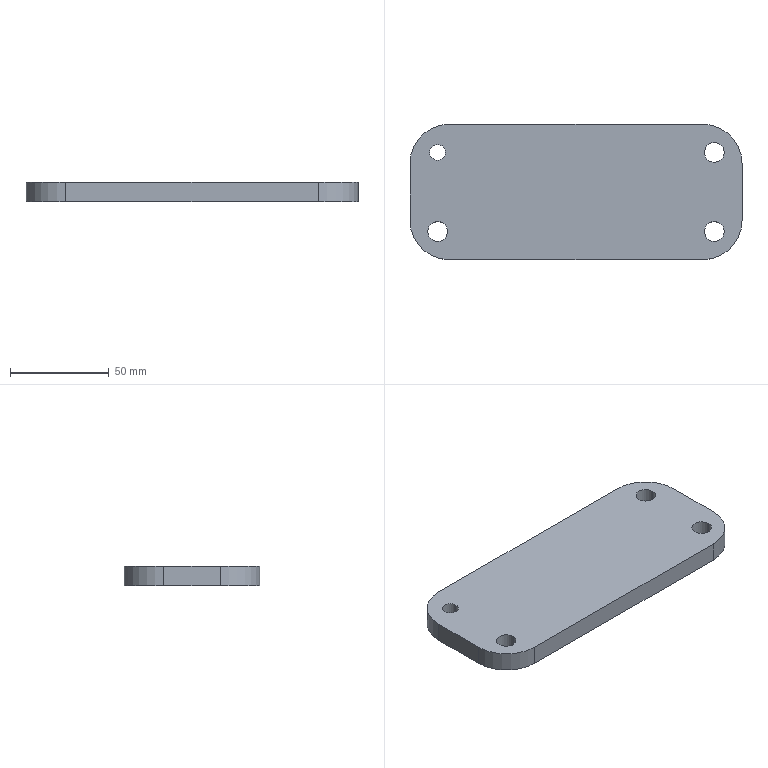Part | SolidWorks | features Cut 1, Extrusion 1, Fillet 1 | 1 solid | 18 faces | box 168 x 68.566 x 10 mm | volume 108898 mm3 | cylinder 12 | plane 6 | commonest cylinder face diameters 10 x6 40 x4 8 x2
STEP:
#1=CARTESIAN_POINT('',(-75.,-100.,-10.));
#2=VERTEX_POINT('',#1);
#3=CARTESIAN_POINT('',(-65.,-100.,-10.));
#4=VERTEX_POINT('',#3);
#5=CARTESIAN_POINT('',(-70.,-100.,-10.));
#6=DIRECTION('',(0.,0.,1.));
#7=DIRECTION('',(1.,0.,0.));
#8=AXIS2_PLACEMENT_3D('',#5,#6,#7);
#9=CIRCLE('',#8,5.);
#10=EDGE_CURVE('',#2,#4,#9,.T.);
#11=ORIENTED_EDGE('',*,*,#10,.F.);
#12=CARTESIAN_POINT('',(-75.,-100.,0.));
#13=VERTEX_POINT('',#12);
#14=CARTESIAN_POINT('',(-75.,-100.,-10.));
#15=DIRECTION('',(0.,0.,1.));
#16=VECTOR('',#15,1000.);
#17=LINE('',#14,#16);
#18=EDGE_CURVE('',#2,#13,#17,.T.);
#19=ORIENTED_EDGE('',*,*,#18,.T.);
#20=CARTESIAN_POINT('',(-65.,-100.,0.));
#21=VERTEX_POINT('',#20);
#22=CARTESIAN_POINT('',(-70.,-100.,0.));
#23=DIRECTION('',(0.,0.,1.));
#24=DIRECTION('',(1.,0.,0.));
#25=AXIS2_PLACEMENT_3D('',#22,#23,#24);
#26=CIRCLE('',#25,5.);
#27=EDGE_CURVE('',#13,#21,#26,.T.);
#28=ORIENTED_EDGE('',*,*,#27,.T.);
#29=CARTESIAN_POINT('',(-65.,-100.,-10.));
#30=DIRECTION('',(0.,0.,1.));
#31=VECTOR('',#30,1000.);
#32=LINE('',#29,#31);
#33=EDGE_CURVE('',#4,#21,#32,.T.);
#34=ORIENTED_EDGE('',*,*,#33,.F.);
#35=EDGE_LOOP('',(#11,#19,#28,#34));
#36=FACE_OUTER_BOUND('',#35,.T.);
#37=CARTESIAN_POINT('',(-70.,-100.,-10.));
#38=DIRECTION('',(0.,0.,1.));
#39=DIRECTION('',(1.,0.,0.));
#40=AXIS2_PLACEMENT_3D('',#37,#38,#39);
#41=CYLINDRICAL_SURFACE('',#40,5.);
#42=ADVANCED_FACE('',(#36),#41,.F.);
#43=CARTESIAN_POINT('',(65.,-60.,-10.));
#44=VERTEX_POINT('',#43);
#45=CARTESIAN_POINT('',(75.,-60.,-10.));
#46=VERTEX_POINT('',#45);
#47=CARTESIAN_POINT('',(70.,-60.,-10.));
#48=DIRECTION('',(0.,0.,1.));
#49=DIRECTION('',(1.,0.,0.));
#50=AXIS2_PLACEMENT_3D('',#47,#48,#49);
#51=CIRCLE('',#50,5.);
#52=EDGE_CURVE('',#44,#46,#51,.T.);
#53=ORIENTED_EDGE('',*,*,#52,.F.);
#54=CARTESIAN_POINT('',(65.,-60.,0.));
#55=VERTEX_POINT('',#54);
#56=CARTESIAN_POINT('',(65.,-60.,-10.));
#57=DIRECTION('',(0.,0.,1.));
#58=VECTOR('',#57,1000.);
#59=LINE('',#56,#58);
#60=EDGE_CURVE('',#44,#55,#59,.T.);
#61=ORIENTED_EDGE('',*,*,#60,.T.);
#62=CARTESIAN_POINT('',(75.,-60.,0.));
#63=VERTEX_POINT('',#62);
#64=CARTESIAN_POINT('',(70.,-60.,0.));
#65=DIRECTION('',(0.,0.,1.));
#66=DIRECTION('',(1.,0.,0.));
#67=AXIS2_PLACEMENT_3D('',#64,#65,#66);
#68=CIRCLE('',#67,5.);
#69=EDGE_CURVE('',#55,#63,#68,.T.);
#70=ORIENTED_EDGE('',*,*,#69,.T.);
#71=CARTESIAN_POINT('',(75.,-60.,-10.));
#72=DIRECTION('',(0.,0.,1.));
#73=VECTOR('',#72,1000.);
#74=LINE('',#71,#73);
#75=EDGE_CURVE('',#46,#63,#74,.T.);
#76=ORIENTED_EDGE('',*,*,#75,.F.);
#77=EDGE_LOOP('',(#53,#61,#70,#76));
#78=FACE_OUTER_BOUND('',#77,.T.);
#79=CARTESIAN_POINT('',(70.,-60.,-10.));
#80=DIRECTION('',(0.,0.,1.));
#81=DIRECTION('',(1.,0.,0.));
#82=AXIS2_PLACEMENT_3D('',#79,#80,#81);
#83=CYLINDRICAL_SURFACE('',#82,5.);
#84=ADVANCED_FACE('',(#78),#83,.F.);
#85=CARTESIAN_POINT('',(65.,-100.,-10.));
#86=VERTEX_POINT('',#85);
#87=CARTESIAN_POINT('',(75.,-100.,-10.));
#88=VERTEX_POINT('',#87);
#89=CARTESIAN_POINT('',(70.,-100.,-10.));
#90=DIRECTION('',(0.,0.,1.));
#91=DIRECTION('',(1.,0.,0.));
#92=AXIS2_PLACEMENT_3D('',#89,#90,#91);
#93=CIRCLE('',#92,5.);
#94=EDGE_CURVE('',#86,#88,#93,.T.);
#95=ORIENTED_EDGE('',*,*,#94,.F.);
#96=CARTESIAN_POINT('',(65.,-100.,0.));
#97=VERTEX_POINT('',#96);
#98=CARTESIAN_POINT('',(65.,-100.,-10.));
#99=DIRECTION('',(0.,0.,1.));
#100=VECTOR('',#99,1000.);
#101=LINE('',#98,#100);
#102=EDGE_CURVE('',#86,#97,#101,.T.);
#103=ORIENTED_EDGE('',*,*,#102,.T.);
#104=CARTESIAN_POINT('',(75.,-100.,0.));
#105=VERTEX_POINT('',#104);
#106=CARTESIAN_POINT('',(70.,-100.,0.));
#107=DIRECTION('',(0.,0.,1.));
#108=DIRECTION('',(1.,0.,0.));
#109=AXIS2_PLACEMENT_3D('',#106,#107,#108);
#110=CIRCLE('',#109,5.);
#111=EDGE_CURVE('',#97,#105,#110,.T.);
#112=ORIENTED_EDGE('',*,*,#111,.T.);
#113=CARTESIAN_POINT('',(75.,-100.,-10.));
#114=DIRECTION('',(0.,0.,1.));
#115=VECTOR('',#114,1000.);
#116=LINE('',#113,#115);
#117=EDGE_CURVE('',#88,#105,#116,.T.);
#118=ORIENTED_EDGE('',*,*,#117,.F.);
#119=EDGE_LOOP('',(#95,#103,#112,#118));
#120=FACE_OUTER_BOUND('',#119,.T.);
#121=CARTESIAN_POINT('',(70.,-100.,-10.));
#122=DIRECTION('',(0.,0.,1.));
#123=DIRECTION('',(1.,0.,0.));
#124=AXIS2_PLACEMENT_3D('',#121,#122,#123);
#125=CYLINDRICAL_SURFACE('',#124,5.);
#126=ADVANCED_FACE('',(#120),#125,.F.);
#127=CARTESIAN_POINT('',(-74.,-60.,-10.));
#128=VERTEX_POINT('',#127);
#129=CARTESIAN_POINT('',(-66.,-60.,-10.));
#130=VERTEX_POINT('',#129);
#131=CARTESIAN_POINT('',(-70.,-60.,-10.));
#132=DIRECTION('',(0.,0.,1.));
#133=DIRECTION('',(1.,0.,0.));
#134=AXIS2_PLACEMENT_3D('',#131,#132,#133);
#135=CIRCLE('',#134,4.);
#136=EDGE_CURVE('',#128,#130,#135,.T.);
#137=ORIENTED_EDGE('',*,*,#136,.F.);
#138=CARTESIAN_POINT('',(-74.,-60.,0.));
#139=VERTEX_POINT('',#138);
#140=CARTESIAN_POINT('',(-74.,-60.,-10.));
#141=DIRECTION('',(0.,0.,1.));
#142=VECTOR('',#141,1000.);
#143=LINE('',#140,#142);
#144=EDGE_CURVE('',#128,#139,#143,.T.);
#145=ORIENTED_EDGE('',*,*,#144,.T.);
#146=CARTESIAN_POINT('',(-66.,-60.,0.));
#147=VERTEX_POINT('',#146);
#148=CARTESIAN_POINT('',(-70.,-60.,0.));
#149=DIRECTION('',(0.,0.,1.));
#150=DIRECTION('',(1.,0.,0.));
#151=AXIS2_PLACEMENT_3D('',#148,#149,#150);
#152=CIRCLE('',#151,4.);
#153=EDGE_CURVE('',#139,#147,#152,.T.);
#154=ORIENTED_EDGE('',*,*,#153,.T.);
#155=CARTESIAN_POINT('',(-66.,-60.,-10.));
#156=DIRECTION('',(0.,0.,1.));
#157=VECTOR('',#156,1000.);
#158=LINE('',#155,#157);
#159=EDGE_CURVE('',#130,#147,#158,.T.);
#160=ORIENTED_EDGE('',*,*,#159,.F.);
#161=EDGE_LOOP('',(#137,#145,#154,#160));
#162=FACE_OUTER_BOUND('',#161,.T.);
#163=CARTESIAN_POINT('',(-70.,-60.,-10.));
#164=DIRECTION('',(0.,0.,1.));
#165=DIRECTION('',(1.,0.,0.));
#166=AXIS2_PLACEMENT_3D('',#163,#164,#165);
#167=CYLINDRICAL_SURFACE('',#166,4.);
#168=ADVANCED_FACE('',(#162),#167,.F.);
#169=CARTESIAN_POINT('',(-84.,-65.717,0.));
#170=VERTEX_POINT('',#169);
#171=CARTESIAN_POINT('',(-84.,-94.283,0.));
#172=VERTEX_POINT('',#171);
#173=CARTESIAN_POINT('',(-84.,-45.717,0.));
#174=DIRECTION('',(0.,-1.,0.));
#175=VECTOR('',#174,1000.);
#176=LINE('',#173,#175);
#177=EDGE_CURVE('',#170,#172,#176,.T.);
#178=ORIENTED_EDGE('',*,*,#177,.F.);
#179=CARTESIAN_POINT('',(-84.,-65.717,-10.));
#180=VERTEX_POINT('',#179);
#181=CARTESIAN_POINT('',(-84.,-65.717,-10.));
#182=DIRECTION('',(0.,0.,-1.));
#183=VECTOR('',#182,1000.);
#184=LINE('',#181,#183);
#185=EDGE_CURVE('',#170,#180,#184,.T.);
#186=ORIENTED_EDGE('',*,*,#185,.T.);
#187=CARTESIAN_POINT('',(-84.,-94.283,-10.));
#188=VERTEX_POINT('',#187);
#189=CARTESIAN_POINT('',(-84.,-45.717,-10.));
#190=DIRECTION('',(0.,-1.,0.));
#191=VECTOR('',#190,1000.);
#192=LINE('',#189,#191);
#193=EDGE_CURVE('',#180,#188,#192,.T.);
#194=ORIENTED_EDGE('',*,*,#193,.T.);
#195=CARTESIAN_POINT('',(-84.,-94.283,-10.));
#196=DIRECTION('',(0.,0.,1.));
#197=VECTOR('',#196,1000.);
#198=LINE('',#195,#197);
#199=EDGE_CURVE('',#188,#172,#198,.T.);
#200=ORIENTED_EDGE('',*,*,#199,.T.);
#201=EDGE_LOOP('',(#178,#186,#194,#200));
#202=FACE_OUTER_BOUND('',#201,.T.);
#203=CARTESIAN_POINT('',(-84.,-45.717,-10.));
#204=DIRECTION('',(-1.,0.,0.));
#205=DIRECTION('',(0.,0.,1.));
#206=AXIS2_PLACEMENT_3D('',#203,#204,#205);
#207=PLANE('',#206);
#208=ADVANCED_FACE('',(#202),#207,.T.);
#209=CARTESIAN_POINT('',(64.,-45.717,-10.));
#210=VERTEX_POINT('',#209);
#211=CARTESIAN_POINT('',(-64.,-45.717,-10.));
#212=VERTEX_POINT('',#211);
#213=CARTESIAN_POINT('',(84.,-45.717,-10.));
#214=DIRECTION('',(-1.,0.,0.));
#215=VECTOR('',#214,1000.);
#216=LINE('',#213,#215);
#217=EDGE_CURVE('',#210,#212,#216,.T.);
#218=ORIENTED_EDGE('',*,*,#217,.T.);
#219=CARTESIAN_POINT('',(-64.,-45.717,0.));
#220=VERTEX_POINT('',#219);
#221=CARTESIAN_POINT('',(-64.,-45.717,-10.));
#222=DIRECTION('',(0.,0.,1.));
#223=VECTOR('',#222,1000.);
#224=LINE('',#221,#223);
#225=EDGE_CURVE('',#212,#220,#224,.T.);
#226=ORIENTED_EDGE('',*,*,#225,.T.);
#227=CARTESIAN_POINT('',(64.,-45.717,0.));
#228=VERTEX_POINT('',#227);
#229=CARTESIAN_POINT('',(84.,-45.717,0.));
#230=DIRECTION('',(-1.,0.,0.));
#231=VECTOR('',#230,1000.);
#232=LINE('',#229,#231);
#233=EDGE_CURVE('',#228,#220,#232,.T.);
#234=ORIENTED_EDGE('',*,*,#233,.F.);
#235=CARTESIAN_POINT('',(64.,-45.717,-10.));
#236=DIRECTION('',(0.,0.,-1.));
#237=VECTOR('',#236,1000.);
#238=LINE('',#235,#237);
#239=EDGE_CURVE('',#228,#210,#238,.T.);
#240=ORIENTED_EDGE('',*,*,#239,.T.);
#241=EDGE_LOOP('',(#218,#226,#234,#240));
#242=FACE_OUTER_BOUND('',#241,.T.);
#243=CARTESIAN_POINT('',(84.,-45.717,-10.));
#244=DIRECTION('',(0.,1.,0.));
#245=DIRECTION('',(0.,0.,1.));
#246=AXIS2_PLACEMENT_3D('',#243,#244,#245);
#247=PLANE('',#246);
#248=ADVANCED_FACE('',(#242),#247,.T.);
#249=CARTESIAN_POINT('',(84.,-94.283,-10.));
#250=VERTEX_POINT('',#249);
#251=CARTESIAN_POINT('',(84.,-65.717,-10.));
#252=VERTEX_POINT('',#251);
#253=CARTESIAN_POINT('',(84.,-45.717,-10.));
#254=DIRECTION('',(0.,1.,0.));
#255=VECTOR('',#254,1000.);
#256=LINE('',#253,#255);
#257=EDGE_CURVE('',#250,#252,#256,.T.);
#258=ORIENTED_EDGE('',*,*,#257,.T.);
#259=CARTESIAN_POINT('',(84.,-65.717,0.));
#260=VERTEX_POINT('',#259);
#261=CARTESIAN_POINT('',(84.,-65.717,-10.));
#262=DIRECTION('',(0.,0.,1.));
#263=VECTOR('',#262,1000.);
#264=LINE('',#261,#263);
#265=EDGE_CURVE('',#252,#260,#264,.T.);
#266=ORIENTED_EDGE('',*,*,#265,.T.);
#267=CARTESIAN_POINT('',(84.,-94.283,0.));
#268=VERTEX_POINT('',#267);
#269=CARTESIAN_POINT('',(84.,-45.717,0.));
#270=DIRECTION('',(0.,1.,0.));
#271=VECTOR('',#270,1000.);
#272=LINE('',#269,#271);
#273=EDGE_CURVE('',#268,#260,#272,.T.);
#274=ORIENTED_EDGE('',*,*,#273,.F.);
#275=CARTESIAN_POINT('',(84.,-94.283,-10.));
#276=DIRECTION('',(0.,0.,-1.));
#277=VECTOR('',#276,1000.);
#278=LINE('',#275,#277);
#279=EDGE_CURVE('',#268,#250,#278,.T.);
#280=ORIENTED_EDGE('',*,*,#279,.T.);
#281=EDGE_LOOP('',(#258,#266,#274,#280));
#282=FACE_OUTER_BOUND('',#281,.T.);
#283=CARTESIAN_POINT('',(84.,-45.717,-10.));
#284=DIRECTION('',(1.,0.,0.));
#285=DIRECTION('',(0.,0.,-1.));
#286=AXIS2_PLACEMENT_3D('',#283,#284,#285);
#287=PLANE('',#286);
#288=ADVANCED_FACE('',(#282),#287,.T.);
#289=CARTESIAN_POINT('',(-64.,-114.283,-10.));
#290=VERTEX_POINT('',#289);
#291=CARTESIAN_POINT('',(64.,-114.283,-10.));
#292=VERTEX_POINT('',#291);
#293=CARTESIAN_POINT('',(84.,-114.283,-10.));
#294=DIRECTION('',(1.,0.,0.));
#295=VECTOR('',#294,1000.);
#296=LINE('',#293,#295);
#297=EDGE_CURVE('',#290,#292,#296,.T.);
#298=ORIENTED_EDGE('',*,*,#297,.T.);
#299=CARTESIAN_POINT('',(64.,-114.283,0.));
#300=VERTEX_POINT('',#299);
#301=CARTESIAN_POINT('',(64.,-114.283,-10.));
#302=DIRECTION('',(0.,0.,1.));
#303=VECTOR('',#302,1000.);
#304=LINE('',#301,#303);
#305=EDGE_CURVE('',#292,#300,#304,.T.);
#306=ORIENTED_EDGE('',*,*,#305,.T.);
#307=CARTESIAN_POINT('',(-64.,-114.283,0.));
#308=VERTEX_POINT('',#307);
#309=CARTESIAN_POINT('',(84.,-114.283,0.));
#310=DIRECTION('',(1.,0.,0.));
#311=VECTOR('',#310,1000.);
#312=LINE('',#309,#311);
#313=EDGE_CURVE('',#308,#300,#312,.T.);
#314=ORIENTED_EDGE('',*,*,#313,.F.);
#315=CARTESIAN_POINT('',(-64.,-114.283,-10.));
#316=DIRECTION('',(0.,0.,-1.));
#317=VECTOR('',#316,1000.);
#318=LINE('',#315,#317);
#319=EDGE_CURVE('',#308,#290,#318,.T.);
#320=ORIENTED_EDGE('',*,*,#319,.T.);
#321=EDGE_LOOP('',(#298,#306,#314,#320));
#322=FACE_OUTER_BOUND('',#321,.T.);
#323=CARTESIAN_POINT('',(84.,-114.283,-10.));
#324=DIRECTION('',(0.,-1.,0.));
#325=DIRECTION('',(0.,0.,-1.));
#326=AXIS2_PLACEMENT_3D('',#323,#324,#325);
#327=PLANE('',#326);
#328=ADVANCED_FACE('',(#322),#327,.T.);
#329=CARTESIAN_POINT('',(-70.,-100.,-10.));
#330=DIRECTION('',(0.,0.,1.));
#331=DIRECTION('',(1.,0.,0.));
#332=AXIS2_PLACEMENT_3D('',#329,#330,#331);
#333=CIRCLE('',#332,5.);
#334=EDGE_CURVE('',#4,#2,#333,.T.);
#335=ORIENTED_EDGE('',*,*,#334,.T.);
#336=ORIENTED_EDGE('',*,*,#10,.T.);
#337=EDGE_LOOP('',(#335,#336));
#338=FACE_BOUND('',#337,.T.);
#339=CARTESIAN_POINT('',(70.,-60.,-10.));
#340=DIRECTION('',(0.,0.,1.));
#341=DIRECTION('',(1.,0.,0.));
#342=AXIS2_PLACEMENT_3D('',#339,#340,#341);
#343=CIRCLE('',#342,5.);
#344=EDGE_CURVE('',#46,#44,#343,.T.);
#345=ORIENTED_EDGE('',*,*,#344,.T.);
#346=ORIENTED_EDGE('',*,*,#52,.T.);
#347=EDGE_LOOP('',(#345,#346));
#348=FACE_BOUND('',#347,.T.);
#349=CARTESIAN_POINT('',(70.,-100.,-10.));
#350=DIRECTION('',(0.,0.,1.));
#351=DIRECTION('',(1.,0.,0.));
#352=AXIS2_PLACEMENT_3D('',#349,#350,#351);
#353=CIRCLE('',#352,5.);
#354=EDGE_CURVE('',#88,#86,#353,.T.);
#355=ORIENTED_EDGE('',*,*,#354,.T.);
#356=ORIENTED_EDGE('',*,*,#94,.T.);
#357=EDGE_LOOP('',(#355,#356));
#358=FACE_BOUND('',#357,.T.);
#359=CARTESIAN_POINT('',(-70.,-60.,-10.));
#360=DIRECTION('',(0.,0.,1.));
#361=DIRECTION('',(1.,0.,0.));
#362=AXIS2_PLACEMENT_3D('',#359,#360,#361);
#363=CIRCLE('',#362,4.);
#364=EDGE_CURVE('',#130,#128,#363,.T.);
#365=ORIENTED_EDGE('',*,*,#364,.T.);
#366=ORIENTED_EDGE('',*,*,#136,.T.);
#367=EDGE_LOOP('',(#365,#366));
#368=FACE_BOUND('',#367,.T.);
#369=ORIENTED_EDGE('',*,*,#193,.F.);
#370=CARTESIAN_POINT('',(-64.,-65.717,-10.));
#371=DIRECTION('',(0.,0.,-1.));
#372=DIRECTION('',(-1.,0.,0.));
#373=AXIS2_PLACEMENT_3D('',#370,#371,#372);
#374=CIRCLE('',#373,20.);
#375=EDGE_CURVE('',#180,#212,#374,.T.);
#376=ORIENTED_EDGE('',*,*,#375,.T.);
#377=ORIENTED_EDGE('',*,*,#217,.F.);
#378=CARTESIAN_POINT('',(64.,-65.717,-10.));
#379=DIRECTION('',(0.,0.,-1.));
#380=DIRECTION('',(-1.,0.,0.));
#381=AXIS2_PLACEMENT_3D('',#378,#379,#380);
#382=CIRCLE('',#381,20.);
#383=EDGE_CURVE('',#210,#252,#382,.T.);
#384=ORIENTED_EDGE('',*,*,#383,.T.);
#385=ORIENTED_EDGE('',*,*,#257,.F.);
#386=CARTESIAN_POINT('',(64.,-94.283,-10.));
#387=DIRECTION('',(0.,0.,-1.));
#388=DIRECTION('',(-1.,0.,0.));
#389=AXIS2_PLACEMENT_3D('',#386,#387,#388);
#390=CIRCLE('',#389,20.);
#391=EDGE_CURVE('',#250,#292,#390,.T.);
#392=ORIENTED_EDGE('',*,*,#391,.T.);
#393=ORIENTED_EDGE('',*,*,#297,.F.);
#394=CARTESIAN_POINT('',(-64.,-94.283,-10.));
#395=DIRECTION('',(0.,0.,-1.));
#396=DIRECTION('',(-1.,0.,0.));
#397=AXIS2_PLACEMENT_3D('',#394,#395,#396);
#398=CIRCLE('',#397,20.);
#399=EDGE_CURVE('',#290,#188,#398,.T.);
#400=ORIENTED_EDGE('',*,*,#399,.T.);
#401=EDGE_LOOP('',(#369,#376,#377,#384,#385,#392,#393,#400));
#402=FACE_OUTER_BOUND('',#401,.T.);
#403=CARTESIAN_POINT('',(0.,0.,-10.));
#404=DIRECTION('',(0.,0.,-1.));
#405=DIRECTION('',(-1.,0.,0.));
#406=AXIS2_PLACEMENT_3D('',#403,#404,#405);
#407=PLANE('',#406);
#408=ADVANCED_FACE('',(#338,#348,#358,#368,#402),#407,.T.);
#409=CARTESIAN_POINT('',(-70.,-100.,0.));
#410=DIRECTION('',(0.,0.,1.));
#411=DIRECTION('',(1.,0.,0.));
#412=AXIS2_PLACEMENT_3D('',#409,#410,#411);
#413=CIRCLE('',#412,5.);
#414=EDGE_CURVE('',#21,#13,#413,.T.);
#415=ORIENTED_EDGE('',*,*,#414,.F.);
#416=ORIENTED_EDGE('',*,*,#27,.F.);
#417=EDGE_LOOP('',(#415,#416));
#418=FACE_BOUND('',#417,.T.);
#419=CARTESIAN_POINT('',(70.,-60.,0.));
#420=DIRECTION('',(0.,0.,1.));
#421=DIRECTION('',(1.,0.,0.));
#422=AXIS2_PLACEMENT_3D('',#419,#420,#421);
#423=CIRCLE('',#422,5.);
#424=EDGE_CURVE('',#63,#55,#423,.T.);
#425=ORIENTED_EDGE('',*,*,#424,.F.);
#426=ORIENTED_EDGE('',*,*,#69,.F.);
#427=EDGE_LOOP('',(#425,#426));
#428=FACE_BOUND('',#427,.T.);
#429=CARTESIAN_POINT('',(70.,-100.,0.));
#430=DIRECTION('',(0.,0.,1.));
#431=DIRECTION('',(1.,0.,0.));
#432=AXIS2_PLACEMENT_3D('',#429,#430,#431);
#433=CIRCLE('',#432,5.);
#434=EDGE_CURVE('',#105,#97,#433,.T.);
#435=ORIENTED_EDGE('',*,*,#434,.F.);
#436=ORIENTED_EDGE('',*,*,#111,.F.);
#437=EDGE_LOOP('',(#435,#436));
#438=FACE_BOUND('',#437,.T.);
#439=CARTESIAN_POINT('',(-70.,-60.,0.));
#440=DIRECTION('',(0.,0.,1.));
#441=DIRECTION('',(1.,0.,0.));
#442=AXIS2_PLACEMENT_3D('',#439,#440,#441);
#443=CIRCLE('',#442,4.);
#444=EDGE_CURVE('',#147,#139,#443,.T.);
#445=ORIENTED_EDGE('',*,*,#444,.F.);
#446=ORIENTED_EDGE('',*,*,#153,.F.);
#447=EDGE_LOOP('',(#445,#446));
#448=FACE_BOUND('',#447,.T.);
#449=ORIENTED_EDGE('',*,*,#233,.T.);
#450=CARTESIAN_POINT('',(-64.,-65.717,0.));
#451=DIRECTION('',(0.,0.,1.));
#452=DIRECTION('',(-1.,0.,0.));
#453=AXIS2_PLACEMENT_3D('',#450,#451,#452);
#454=CIRCLE('',#453,20.);
#455=EDGE_CURVE('',#220,#170,#454,.T.);
#456=ORIENTED_EDGE('',*,*,#455,.T.);
#457=ORIENTED_EDGE('',*,*,#177,.T.);
#458=CARTESIAN_POINT('',(-64.,-94.283,0.));
#459=DIRECTION('',(0.,0.,1.));
#460=DIRECTION('',(-1.,0.,0.));
#461=AXIS2_PLACEMENT_3D('',#458,#459,#460);
#462=CIRCLE('',#461,20.);
#463=EDGE_CURVE('',#172,#308,#462,.T.);
#464=ORIENTED_EDGE('',*,*,#463,.T.);
#465=ORIENTED_EDGE('',*,*,#313,.T.);
#466=CARTESIAN_POINT('',(64.,-94.283,0.));
#467=DIRECTION('',(0.,0.,1.));
#468=DIRECTION('',(-1.,0.,0.));
#469=AXIS2_PLACEMENT_3D('',#466,#467,#468);
#470=CIRCLE('',#469,20.);
#471=EDGE_CURVE('',#300,#268,#470,.T.);
#472=ORIENTED_EDGE('',*,*,#471,.T.);
#473=ORIENTED_EDGE('',*,*,#273,.T.);
#474=CARTESIAN_POINT('',(64.,-65.717,0.));
#475=DIRECTION('',(0.,0.,1.));
#476=DIRECTION('',(-1.,0.,0.));
#477=AXIS2_PLACEMENT_3D('',#474,#475,#476);
#478=CIRCLE('',#477,20.);
#479=EDGE_CURVE('',#260,#228,#478,.T.);
#480=ORIENTED_EDGE('',*,*,#479,.T.);
#481=EDGE_LOOP('',(#449,#456,#457,#464,#465,#472,#473,#480));
#482=FACE_OUTER_BOUND('',#481,.T.);
#483=CARTESIAN_POINT('',(0.,0.,0.));
#484=DIRECTION('',(0.,0.,-1.));
#485=DIRECTION('',(-1.,0.,0.));
#486=AXIS2_PLACEMENT_3D('',#483,#484,#485);
#487=PLANE('',#486);
#488=ADVANCED_FACE('',(#418,#428,#438,#448,#482),#487,.F.);
#489=ORIENTED_EDGE('',*,*,#144,.F.);
#490=ORIENTED_EDGE('',*,*,#364,.F.);
#491=ORIENTED_EDGE('',*,*,#159,.T.);
#492=ORIENTED_EDGE('',*,*,#444,.T.);
#493=EDGE_LOOP('',(#489,#490,#491,#492));
#494=FACE_OUTER_BOUND('',#493,.T.);
#495=CARTESIAN_POINT('',(-70.,-60.,-10.));
#496=DIRECTION('',(0.,0.,1.));
#497=DIRECTION('',(1.,0.,0.));
#498=AXIS2_PLACEMENT_3D('',#495,#496,#497);
#499=CYLINDRICAL_SURFACE('',#498,4.);
#500=ADVANCED_FACE('',(#494),#499,.F.);
#501=ORIENTED_EDGE('',*,*,#102,.F.);
#502=ORIENTED_EDGE('',*,*,#354,.F.);
#503=ORIENTED_EDGE('',*,*,#117,.T.);
#504=ORIENTED_EDGE('',*,*,#434,.T.);
#505=EDGE_LOOP('',(#501,#502,#503,#504));
#506=FACE_OUTER_BOUND('',#505,.T.);
#507=CARTESIAN_POINT('',(70.,-100.,-10.));
#508=DIRECTION('',(0.,0.,1.));
#509=DIRECTION('',(1.,0.,0.));
#510=AXIS2_PLACEMENT_3D('',#507,#508,#509);
#511=CYLINDRICAL_SURFACE('',#510,5.);
#512=ADVANCED_FACE('',(#506),#511,.F.);
#513=ORIENTED_EDGE('',*,*,#60,.F.);
#514=ORIENTED_EDGE('',*,*,#344,.F.);
#515=ORIENTED_EDGE('',*,*,#75,.T.);
#516=ORIENTED_EDGE('',*,*,#424,.T.);
#517=EDGE_LOOP('',(#513,#514,#515,#516));
#518=FACE_OUTER_BOUND('',#517,.T.);
#519=CARTESIAN_POINT('',(70.,-60.,-10.));
#520=DIRECTION('',(0.,0.,1.));
#521=DIRECTION('',(1.,0.,0.));
#522=AXIS2_PLACEMENT_3D('',#519,#520,#521);
#523=CYLINDRICAL_SURFACE('',#522,5.);
#524=ADVANCED_FACE('',(#518),#523,.F.);
#525=ORIENTED_EDGE('',*,*,#18,.F.);
#526=ORIENTED_EDGE('',*,*,#334,.F.);
#527=ORIENTED_EDGE('',*,*,#33,.T.);
#528=ORIENTED_EDGE('',*,*,#414,.T.);
#529=EDGE_LOOP('',(#525,#526,#527,#528));
#530=FACE_OUTER_BOUND('',#529,.T.);
#531=CARTESIAN_POINT('',(-70.,-100.,-10.));
#532=DIRECTION('',(0.,0.,1.));
#533=DIRECTION('',(1.,0.,0.));
#534=AXIS2_PLACEMENT_3D('',#531,#532,#533);
#535=CYLINDRICAL_SURFACE('',#534,5.);
#536=ADVANCED_FACE('',(#530),#535,.F.);
#537=ORIENTED_EDGE('',*,*,#375,.F.);
#538=ORIENTED_EDGE('',*,*,#185,.F.);
#539=ORIENTED_EDGE('',*,*,#455,.F.);
#540=ORIENTED_EDGE('',*,*,#225,.F.);
#541=EDGE_LOOP('',(#537,#538,#539,#540));
#542=FACE_OUTER_BOUND('',#541,.T.);
#543=CARTESIAN_POINT('',(-64.,-65.717,-10.));
#544=DIRECTION('',(0.,0.,1.));
#545=DIRECTION('',(1.,0.,0.));
#546=AXIS2_PLACEMENT_3D('',#543,#544,#545);
#547=CYLINDRICAL_SURFACE('',#546,20.);
#548=ADVANCED_FACE('',(#542),#547,.T.);
#549=ORIENTED_EDGE('',*,*,#383,.F.);
#550=ORIENTED_EDGE('',*,*,#239,.F.);
#551=ORIENTED_EDGE('',*,*,#479,.F.);
#552=ORIENTED_EDGE('',*,*,#265,.F.);
#553=EDGE_LOOP('',(#549,#550,#551,#552));
#554=FACE_OUTER_BOUND('',#553,.T.);
#555=CARTESIAN_POINT('',(64.,-65.717,-10.));
#556=DIRECTION('',(0.,0.,1.));
#557=DIRECTION('',(1.,0.,0.));
#558=AXIS2_PLACEMENT_3D('',#555,#556,#557);
#559=CYLINDRICAL_SURFACE('',#558,20.);
#560=ADVANCED_FACE('',(#554),#559,.T.);
#561=ORIENTED_EDGE('',*,*,#391,.F.);
#562=ORIENTED_EDGE('',*,*,#279,.F.);
#563=ORIENTED_EDGE('',*,*,#471,.F.);
#564=ORIENTED_EDGE('',*,*,#305,.F.);
#565=EDGE_LOOP('',(#561,#562,#563,#564));
#566=FACE_OUTER_BOUND('',#565,.T.);
#567=CARTESIAN_POINT('',(64.,-94.283,-10.));
#568=DIRECTION('',(0.,0.,1.));
#569=DIRECTION('',(1.,0.,0.));
#570=AXIS2_PLACEMENT_3D('',#567,#568,#569);
#571=CYLINDRICAL_SURFACE('',#570,20.);
#572=ADVANCED_FACE('',(#566),#571,.T.);
#573=ORIENTED_EDGE('',*,*,#399,.F.);
#574=ORIENTED_EDGE('',*,*,#319,.F.);
#575=ORIENTED_EDGE('',*,*,#463,.F.);
#576=ORIENTED_EDGE('',*,*,#199,.F.);
#577=EDGE_LOOP('',(#573,#574,#575,#576));
#578=FACE_OUTER_BOUND('',#577,.T.);
#579=CARTESIAN_POINT('',(-64.,-94.283,-10.));
#580=DIRECTION('',(0.,0.,1.));
#581=DIRECTION('',(1.,0.,0.));
#582=AXIS2_PLACEMENT_3D('',#579,#580,#581);
#583=CYLINDRICAL_SURFACE('',#582,20.);
#584=ADVANCED_FACE('',(#578),#583,.T.);
#585=CLOSED_SHELL('',(#42,#84,#126,#168,#208,#248,#288,#328,#408,#488,#500,#512,#524,#536,#548,#560,#572,#584));
#586=MANIFOLD_SOLID_BREP('',#585);
#587=CARTESIAN_POINT('',(0.,0.,0.));
#588=DIRECTION('',(0.,0.,1.));
#589=DIRECTION('',(1.,0.,0.));
#590=AXIS2_PLACEMENT_3D('',#587,#588,#589);
#591=(LENGTH_UNIT()NAMED_UNIT(*)SI_UNIT(.MILLI.,.METRE.));
#592=UNCERTAINTY_MEASURE_WITH_UNIT(LENGTH_MEASURE(0.00001),#591,'','');
#593=(NAMED_UNIT(*)PLANE_ANGLE_UNIT()SI_UNIT($,.RADIAN.));
#594=(NAMED_UNIT(*)SI_UNIT($,.STERADIAN.)SOLID_ANGLE_UNIT());
#595=(GEOMETRIC_REPRESENTATION_CONTEXT(3)GLOBAL_UNCERTAINTY_ASSIGNED_CONTEXT((#592))GLOBAL_UNIT_ASSIGNED_CONTEXT((#591,#593,#594))REPRESENTATION_CONTEXT('',''));
#596=ADVANCED_BREP_SHAPE_REPRESENTATION('',(#586,#590),#595);